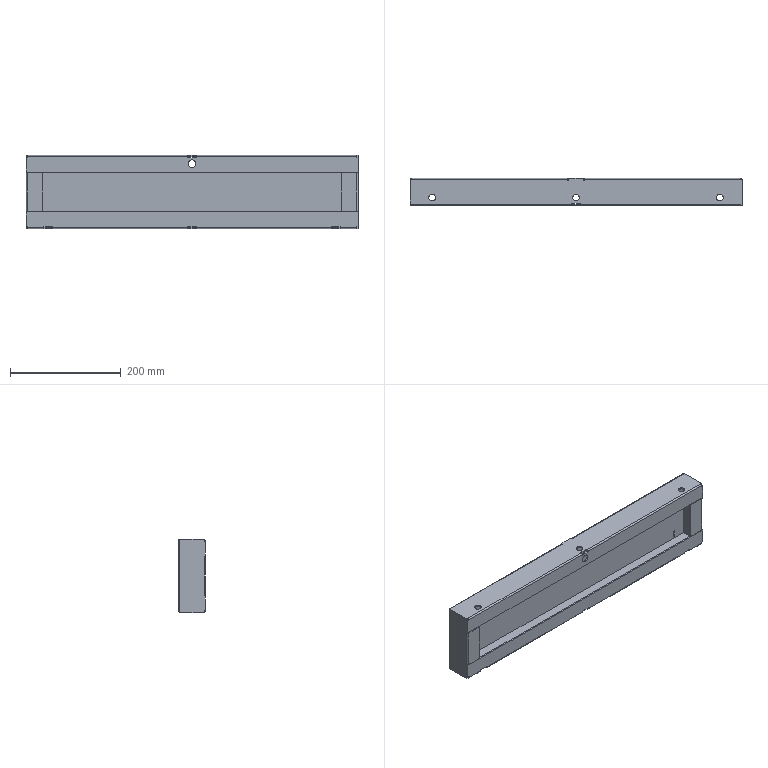Part | NX | features solid 2 | 1 solid | 119 faces | box 600 x 48.71 x 132 mm | volume 448519 mm3 | plane 84 | cylinder 31 | spline 4 | commonest cylinder face diameters 5 x13 12 x12 4 x2 10 x2 14 x2